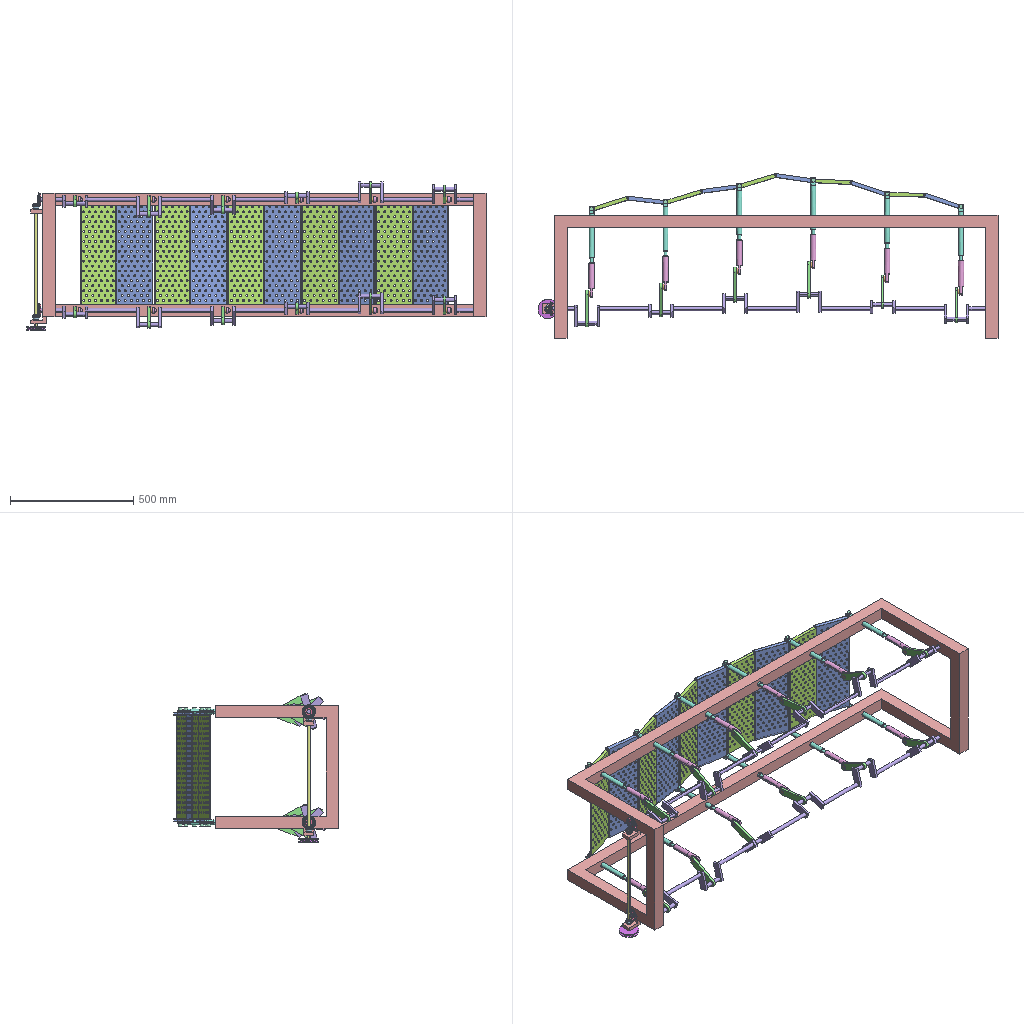Assembly | SolidWorks | 15 different items | 92 placed | box 1868 x 669 x 604 mm
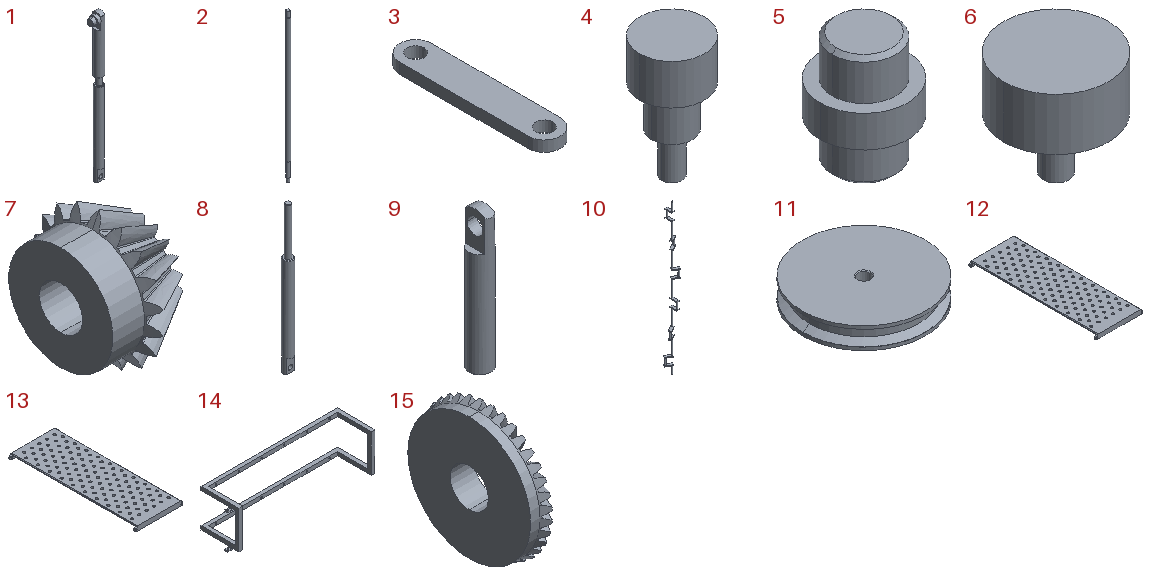Parts list (item | name | quantity | parent item | size | volume | features):
1 | (subassembly) | x12 | - | 34 x 22 x 369.866 mm | 116045 mm3 | -
2 | - | x1 | - | 14 x 14 x 516 mm | 72599 mm3 | features ICE 3, Extrusion 1
3 | - | x12 | - | 30 x 150 x 10 mm | 39047 mm3 | features Extrusion 1
4 | - | x12 | - | 16 x 16 x 30 mm | 2992 mm3 | features ICE 2, Extrusion 1
5 | - | x12 | in 1 | 22 x 22 x 28 mm | 7014 mm3 | features ICE 2, Chamfer 1, Extrusion 1
6 | - | x1 | - | 20 x 20 x 20 mm | 3338 mm3 | features Extrusion 1, ICE 1
7 | - | x2 | - | 19.27 x 30.102 x 30.566 mm | 6238 mm3 | features CirPattern 2, Cut 2, BlendCut 1, Boss 1, ICE 1, Revolution 1
8 | - | x12 | in 1 | 20 x 20 x 310 mm | 72765 mm3 | features ICE 3, Chamfer 1, Extrusion 1
9 | - | x12 | in 1 | 22 x 22 x 139.866 mm | 36266 mm3 | features ICE 2, 3DProfileFeature 1, Chamfer 1, Extrusion 1, HoleWzd 1
10 | - | x2 | - | 136.244 x 140 x 1800 mm | 625784 mm3 | features ICE 24, Extrusion 1
11 | - | x1 | - | 80 x 80 x 14 mm | 61206 mm3 | features Chamfer 1, Extrusion 1, RevCut 1
12 | - | x5 | - | 163 x 440 x 15 mm | 316227 mm3 | features ICE 4, Chamfer 1, Extrusion 1, Fillet 1, LPattern 1
13 | - | x5 | - | 163 x 430 x 15 mm | 308772 mm3 | features ICE 4, Chamfer 1, Extrusion 1, Fillet 1, LPattern 1
14 | - | x1 | - | 1848 x 500 x 530 mm | 15360816 mm3 | features ICE 11, Extrusion 1, LPattern 1
15 | - | x2 | - | 12.396 x 54.775 x 54.775 mm | 17958 mm3 | features CirPattern 2, Cut 2, BlendCut 1, Boss 1, ICE 1, Revolution 1
Mates (type | each side: item.copy, entity, surface, feature):
In the top assembly
Concentric | 12.1 face cylinder Cut-Extrude2 | 13.1 face cylinder Cut-Extrude2
Coincident | 12.1 face plane Boss-Extrude2 | 13.1 face plane Boss-Extrude2
Concentric | 13.1 face cylinder Cut-Extrude2 | 12.2 face cylinder Cut-Extrude2
Coincident | 12.1 face plane Boss-Extrude2 | 12.2 face plane Boss-Extrude2
Coincident | 13.1 face plane Boss-Extrude2 | 13.2 face plane Boss-Extrude2
Concentric | 12.2 face cylinder Cut-Extrude2 | 13.2 face cylinder Cut-Extrude2
Coincident | 12.2 face plane Boss-Extrude2 | 12.3 face plane Boss-Extrude2
Concentric | 13.2 face cylinder Cut-Extrude2 | 12.3 face cylinder Cut-Extrude2
Coincident | 13.2 face plane Boss-Extrude2 | 13.3 face plane Boss-Extrude2
Coincident | 12.3 face plane Boss-Extrude2 | 12.4 face plane Boss-Extrude2
Concentric | 13.3 face cylinder Cut-Extrude2 | 12.4 face cylinder Cut-Extrude2
Coincident | 13.3 face plane Boss-Extrude2 | 13.4 face plane Boss-Extrude2
Concentric | 13.4 face cylinder Cut-Extrude2 | 12.5 face cylinder Cut-Extrude2
Coincident | 12.4 face plane Boss-Extrude2 | 12.5 face plane Boss-Extrude2
Concentric | 12.5 face cylinder Cut-Extrude2 | 13.5 face cylinder Cut-Extrude2
Coincident | 13.4 face plane Boss-Extrude2 | 13.5 face plane Boss-Extrude2
Concentric | 14.1 face cylinder Cut-Extrude2 | 10.1 face cylinder Boss-Extrude25
Concentric | 10.1 face cylinder Boss-Extrude2 | 3.1 face cylinder Boss-Extrude1
DistanceDim | 3.1 face plane Boss-Extrude1 | 10.1 face plane Boss-Extrude1
Concentric | 10.1 face cylinder Boss-Extrude6 | 3.2 face cylinder Boss-Extrude1
DistanceDim | 3.2 face plane Boss-Extrude1 | 10.1 face plane Boss-Extrude5
Concentric | 10.1 face cylinder Boss-Extrude10 | 3.3 face cylinder Boss-Extrude1
DistanceDim | 3.3 face plane Boss-Extrude1 | 10.1 face plane Boss-Extrude9
Concentric | 10.1 face cylinder Boss-Extrude14 | 3.4 face cylinder Boss-Extrude1
DistanceDim | 3.4 face plane Boss-Extrude1 | 10.1 face plane Boss-Extrude13
Concentric | 10.1 face cylinder Boss-Extrude18 | 3.5 face cylinder Boss-Extrude1
DistanceDim | 3.5 face plane Boss-Extrude1 | 10.1 face plane Boss-Extrude17
Concentric | 10.1 face cylinder Boss-Extrude22 | 3.6 face cylinder Boss-Extrude1
DistanceDim | 10.1 face plane Boss-Extrude1 | 14.1 face plane Boss-Extrude1
DistanceDim | 10.1 face plane Boss-Extrude21 | 3.6 face plane Boss-Extrude1
DistanceDim | 13.5 face plane Boss-Extrude3 | 14.1 face plane Boss-Extrude1
Concentric | 14.1 face cylinder Cut-Extrude2 | 10.2 face cylinder Boss-Extrude24
Coincident | 10.1 face plane Boss-Extrude1 | 10.2 face plane Boss-Extrude23
Concentric | 10.2 face cylinder Boss-Extrude22 | 3.7 face cylinder Boss-Extrude1
DistanceDim | 3.7 face plane Boss-Extrude1 | 10.2 face plane Boss-Extrude23
Concentric | 10.2 face cylinder Boss-Extrude18 | 3.8 face cylinder Boss-Extrude1
DistanceDim | 3.8 face plane Boss-Extrude1 | 10.2 face plane Boss-Extrude19
Concentric | 10.2 face cylinder Boss-Extrude14 | 3.9 face cylinder Boss-Extrude1
DistanceDim | 3.9 face plane Boss-Extrude1 | 10.2 face plane Boss-Extrude15
Concentric | 10.2 face cylinder Boss-Extrude10 | 3.10 face cylinder Boss-Extrude1
DistanceDim | 3.10 face plane Boss-Extrude1 | 10.2 face plane Boss-Extrude11
Concentric | 10.2 face cylinder Boss-Extrude6 | 3.11 face cylinder Boss-Extrude1
DistanceDim | 3.11 face plane Boss-Extrude1 | 10.2 face plane Boss-Extrude7
Concentric | 10.2 face cylinder Boss-Extrude2 | 3.12 face cylinder Boss-Extrude1
DistanceDim | 3.12 face plane Boss-Extrude1 | 10.2 face plane Boss-Extrude3
Concentric | 12.4 face cylinder Cut-Extrude2 | 13.4 face cylinder Cut-Extrude2
Concentric | 12.3 face cylinder Cut-Extrude2 | 13.3 face cylinder Cut-Extrude2
Concentric | 10.1 face cylinder Boss-Extrude25 | 15.1 face cylinder Cut-Extrude2
Coincident | 10.1 face plane Boss-Extrude25 | 15.1 face plane Base-Revolve
Concentric | 10.2 face cylinder Boss-Extrude24 | 15.2 face cylinder Cut-Extrude2
Coincident | 10.2 face plane Boss-Extrude24 | 15.2 face plane Base-Revolve
Concentric | 7.1 face cylinder Cut-Extrude1 | 2.1 face cylinder Boss-Extrude2
Coincident | 7.1 face plane Hub | 2.1 face plane Boss-Extrude1
Concentric | 14.1 face cylinder Cut-Extrude3 | 2.1 face cylinder Boss-Extrude2
DistanceDim | 7.1 face plane Hub | 14.1 face plane Boss-Extrude8
Concentric | 2.1 face cylinder Boss-Extrude3 | 7.2 face cylinder Hub
DistanceDim | 7.2 face plane Hub | 14.1 face plane Boss-Extrude8
Concentric | 2.1 face cylinder Boss-Extrude4 | 11.1 face cylinder Boss-Extrude1
Coincident | 2.1 face plane Boss-Extrude3 | 11.1 face plane Boss-Extrude1
GearDim | 15.2 face cone Base-Revolve | 7.2 face cone Base-Revolve
Concentric | 14.1 face cylinder Cut-Extrude1 | 8.1 face cylinder Boss-Extrude1
Coincident | 8.1 face plane Cut-Extrude2 | 4.1 face plane Boss-Extrude3
Concentric | 8.1 face cylinder Cut-Extrude1 | 4.1 face cylinder Boss-Extrude1
Concentric | 13.5 face cylinder Cut-Extrude2 | 4.1 face cylinder Boss-Extrude1
Concentric | 9.1 face cylinder Cut-Extrude2 | 3.7 face cylinder Boss-Extrude1
Concentric | 4.2 face cylinder Boss-Extrude2 | 8.2 face cylinder Cut-Extrude1
Concentric | 14.1 face cylinder LPattern1 | 8.2 face cylinder Boss-Extrude1
Concentric | 3.8 face cylinder Boss-Extrude1 | 5.1 face cylinder Boss-Extrude3
Concentric | 13.4 face cylinder Cut-Extrude2 | 4.2 face cylinder Boss-Extrude1
Concentric | 4.3 face cylinder Boss-Extrude2 | 8.3 face cylinder Cut-Extrude1
Concentric | 14.1 face cylinder LPattern1 | 8.3 face cylinder Boss-Extrude1
Concentric | 3.9 face cylinder Boss-Extrude1 | 5.2 face cylinder Boss-Extrude3
Concentric | 4.4 face cylinder Boss-Extrude2 | 8.4 face cylinder Cut-Extrude1
Concentric | 14.1 face cylinder LPattern1 | 8.4 face cylinder Boss-Extrude1
Concentric | 3.10 face cylinder Boss-Extrude1 | 5.3 face cylinder Boss-Extrude3
Concentric | 4.5 face cylinder Boss-Extrude2 | 8.5 face cylinder Cut-Extrude1
Concentric | 14.1 face cylinder LPattern1 | 8.5 face cylinder Boss-Extrude1
Concentric | 3.11 face cylinder Boss-Extrude1 | 5.4 face cylinder Boss-Extrude3
Concentric | 4.6 face cylinder Boss-Extrude2 | 8.6 face cylinder Cut-Extrude1
Concentric | 14.1 face cylinder LPattern1 | 8.6 face cylinder Boss-Extrude1
Concentric | 3.12 face cylinder Boss-Extrude1 | 5.5 face cylinder Boss-Extrude3
Concentric | 12.4 face cylinder Cut-Extrude2 | 4.3 face cylinder Boss-Extrude1
Concentric | 12.3 face cylinder Cut-Extrude2 | 4.4 face cylinder Boss-Extrude1
Concentric | 12.2 face cylinder Cut-Extrude2 | 4.5 face cylinder Boss-Extrude1
Concentric | 12.1 face cylinder Cut-Extrude2 | 4.6 face cylinder Boss-Extrude1
Coincident | 4.6 face plane Boss-Extrude3 | 8.6 face plane Cut-Extrude2
Coincident | 4.5 face plane Boss-Extrude3 | 8.5 face plane Cut-Extrude2
Coincident | 4.3 face plane Boss-Extrude3 | 8.3 face plane Cut-Extrude2
Coincident | 4.3 face plane Boss-Extrude3 | 4.4 face plane Boss-Extrude3
Coincident | 4.2 face plane Boss-Extrude3 | 4.3 face plane Boss-Extrude3
Concentric | 14.1 face cylinder Cut-Extrude1 | 8.7 face cylinder Boss-Extrude1
Concentric | 4.7 face cylinder Boss-Extrude2 | 8.7 face cylinder Cut-Extrude1
Concentric | 3.1 face cylinder Boss-Extrude1 | 5.6 face cylinder Boss-Extrude3
Coincident | 4.7 face plane Boss-Extrude3 | 8.7 face plane Cut-Extrude2
Concentric | 13.5 face cylinder Cut-Extrude2 | 8.7 face cylinder Cut-Extrude1
Concentric | 14.1 face cylinder LPattern1 | 8.8 face cylinder Boss-Extrude1
Concentric | 4.8 face cylinder Boss-Extrude2 | 8.8 face cylinder Cut-Extrude1
Concentric | 3.2 face cylinder Boss-Extrude1 | 5.7 face cylinder Boss-Extrude3
Coincident | 4.8 face plane Boss-Extrude3 | 8.8 face plane Cut-Extrude2
Concentric | 4.2 face cylinder Boss-Extrude3 | 8.8 face cylinder Cut-Extrude1
Concentric | 14.1 face cylinder LPattern1 | 8.9 face cylinder Boss-Extrude1
Concentric | 4.9 face cylinder Boss-Extrude2 | 8.9 face cylinder Cut-Extrude1
Concentric | 3.3 face cylinder Boss-Extrude1 | 5.8 face cylinder Boss-Extrude3
Coincident | 4.9 face plane Boss-Extrude3 | 8.9 face plane Cut-Extrude2
Concentric | 4.3 face cylinder Boss-Extrude3 | 8.9 face cylinder Cut-Extrude1
Concentric | 14.1 face cylinder LPattern1 | 8.10 face cylinder Boss-Extrude1
Concentric | 4.10 face cylinder Boss-Extrude2 | 8.10 face cylinder Cut-Extrude1
Concentric | 3.4 face cylinder Boss-Extrude1 | 5.9 face cylinder Boss-Extrude3
Coincident | 4.10 face plane Boss-Extrude3 | 8.10 face plane Cut-Extrude2
Concentric | 4.4 face cylinder Boss-Extrude3 | 8.10 face cylinder Cut-Extrude1
Concentric | 14.1 face cylinder LPattern1 | 8.11 face cylinder Boss-Extrude1
Concentric | 4.11 face cylinder Boss-Extrude3 | 8.11 face cylinder Cut-Extrude1
Concentric | 3.5 face cylinder Boss-Extrude1 | 5.10 face cylinder Boss-Extrude3
Coincident | 4.11 face plane Boss-Extrude3 | 8.11 face plane Cut-Extrude2
Concentric | 4.5 face cylinder Boss-Extrude3 | 8.11 face cylinder Cut-Extrude1
Concentric | 14.1 face cylinder LPattern1 | 8.12 face cylinder Boss-Extrude1
Concentric | 4.12 face cylinder Boss-Extrude3 | 8.12 face cylinder Cut-Extrude1
Concentric | 3.6 face cylinder Boss-Extrude1 | 5.11 face cylinder Boss-Extrude3
Coincident | 4.12 face plane Boss-Extrude3 | 8.12 face plane Cut-Extrude2
Concentric | 4.6 face cylinder Boss-Extrude3 | 8.12 face cylinder Cut-Extrude1
In subassembly 1
Concentric | 9.2 face cylinder Boss-Extrude1 | 8.13 face cylinder Boss-Extrude2
DistanceDim | 8.13 face plane Boss-Extrude1 | 9.2 face plane Boss-Extrude1
Perpendicular | 9.2 face plane Cut-Extrude1 | 8.13 face plane Cut-Extrude2
Concentric | 9.2 face cylinder Cut-Extrude2 | 5.12 face cylinder Boss-Extrude3
Coincident | 9.2 face plane Cut-Extrude1 | 5.12 face plane Boss-Extrude2